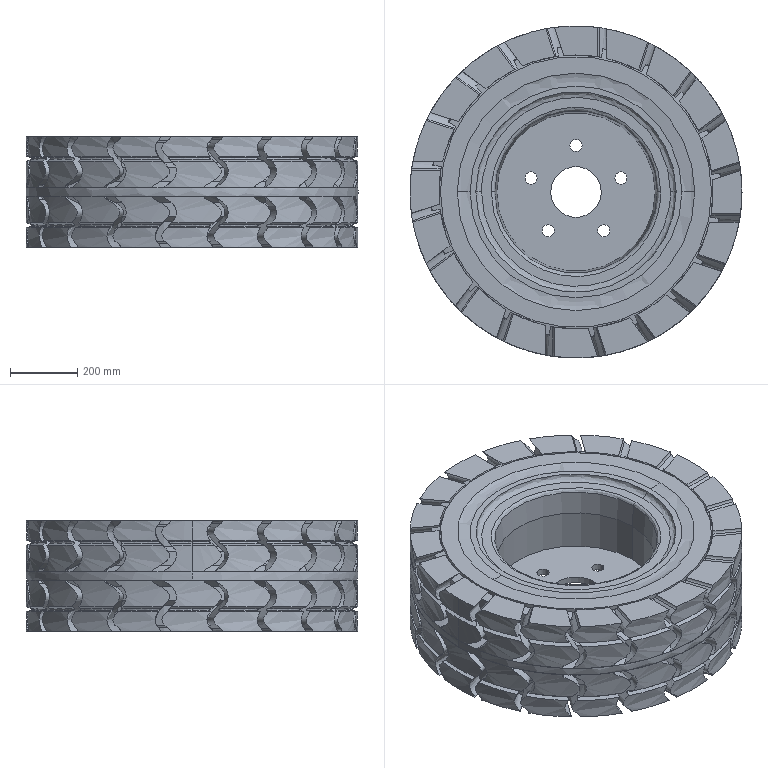Part | SolidWorks | features BaseBody 42 | 42 solids | 757 faces | box 984.493 x 984.493 x 328 mm | volume 181594860 mm3 | cylinder 322 | cone 231 | spline 152 | plane 52 | commonest cylinder face diameters 984 x84 20 x80 864 x46 916 x46 812 x42 36 x10